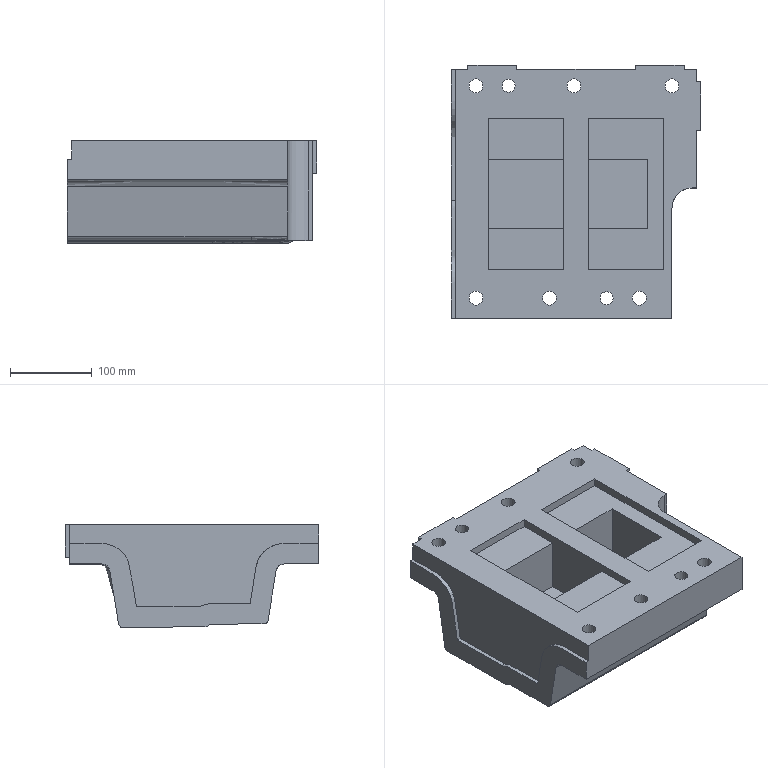Part | NX | features solid 2 | 1 solid | 142 faces | box 305 x 310 x 125.996 mm | volume 6829711 mm3 | plane 57 | spline 57 | cylinder 28 | commonest cylinder face diameters 17 x6 26 x6 12 x4 10 x3 9 x2 16 x2